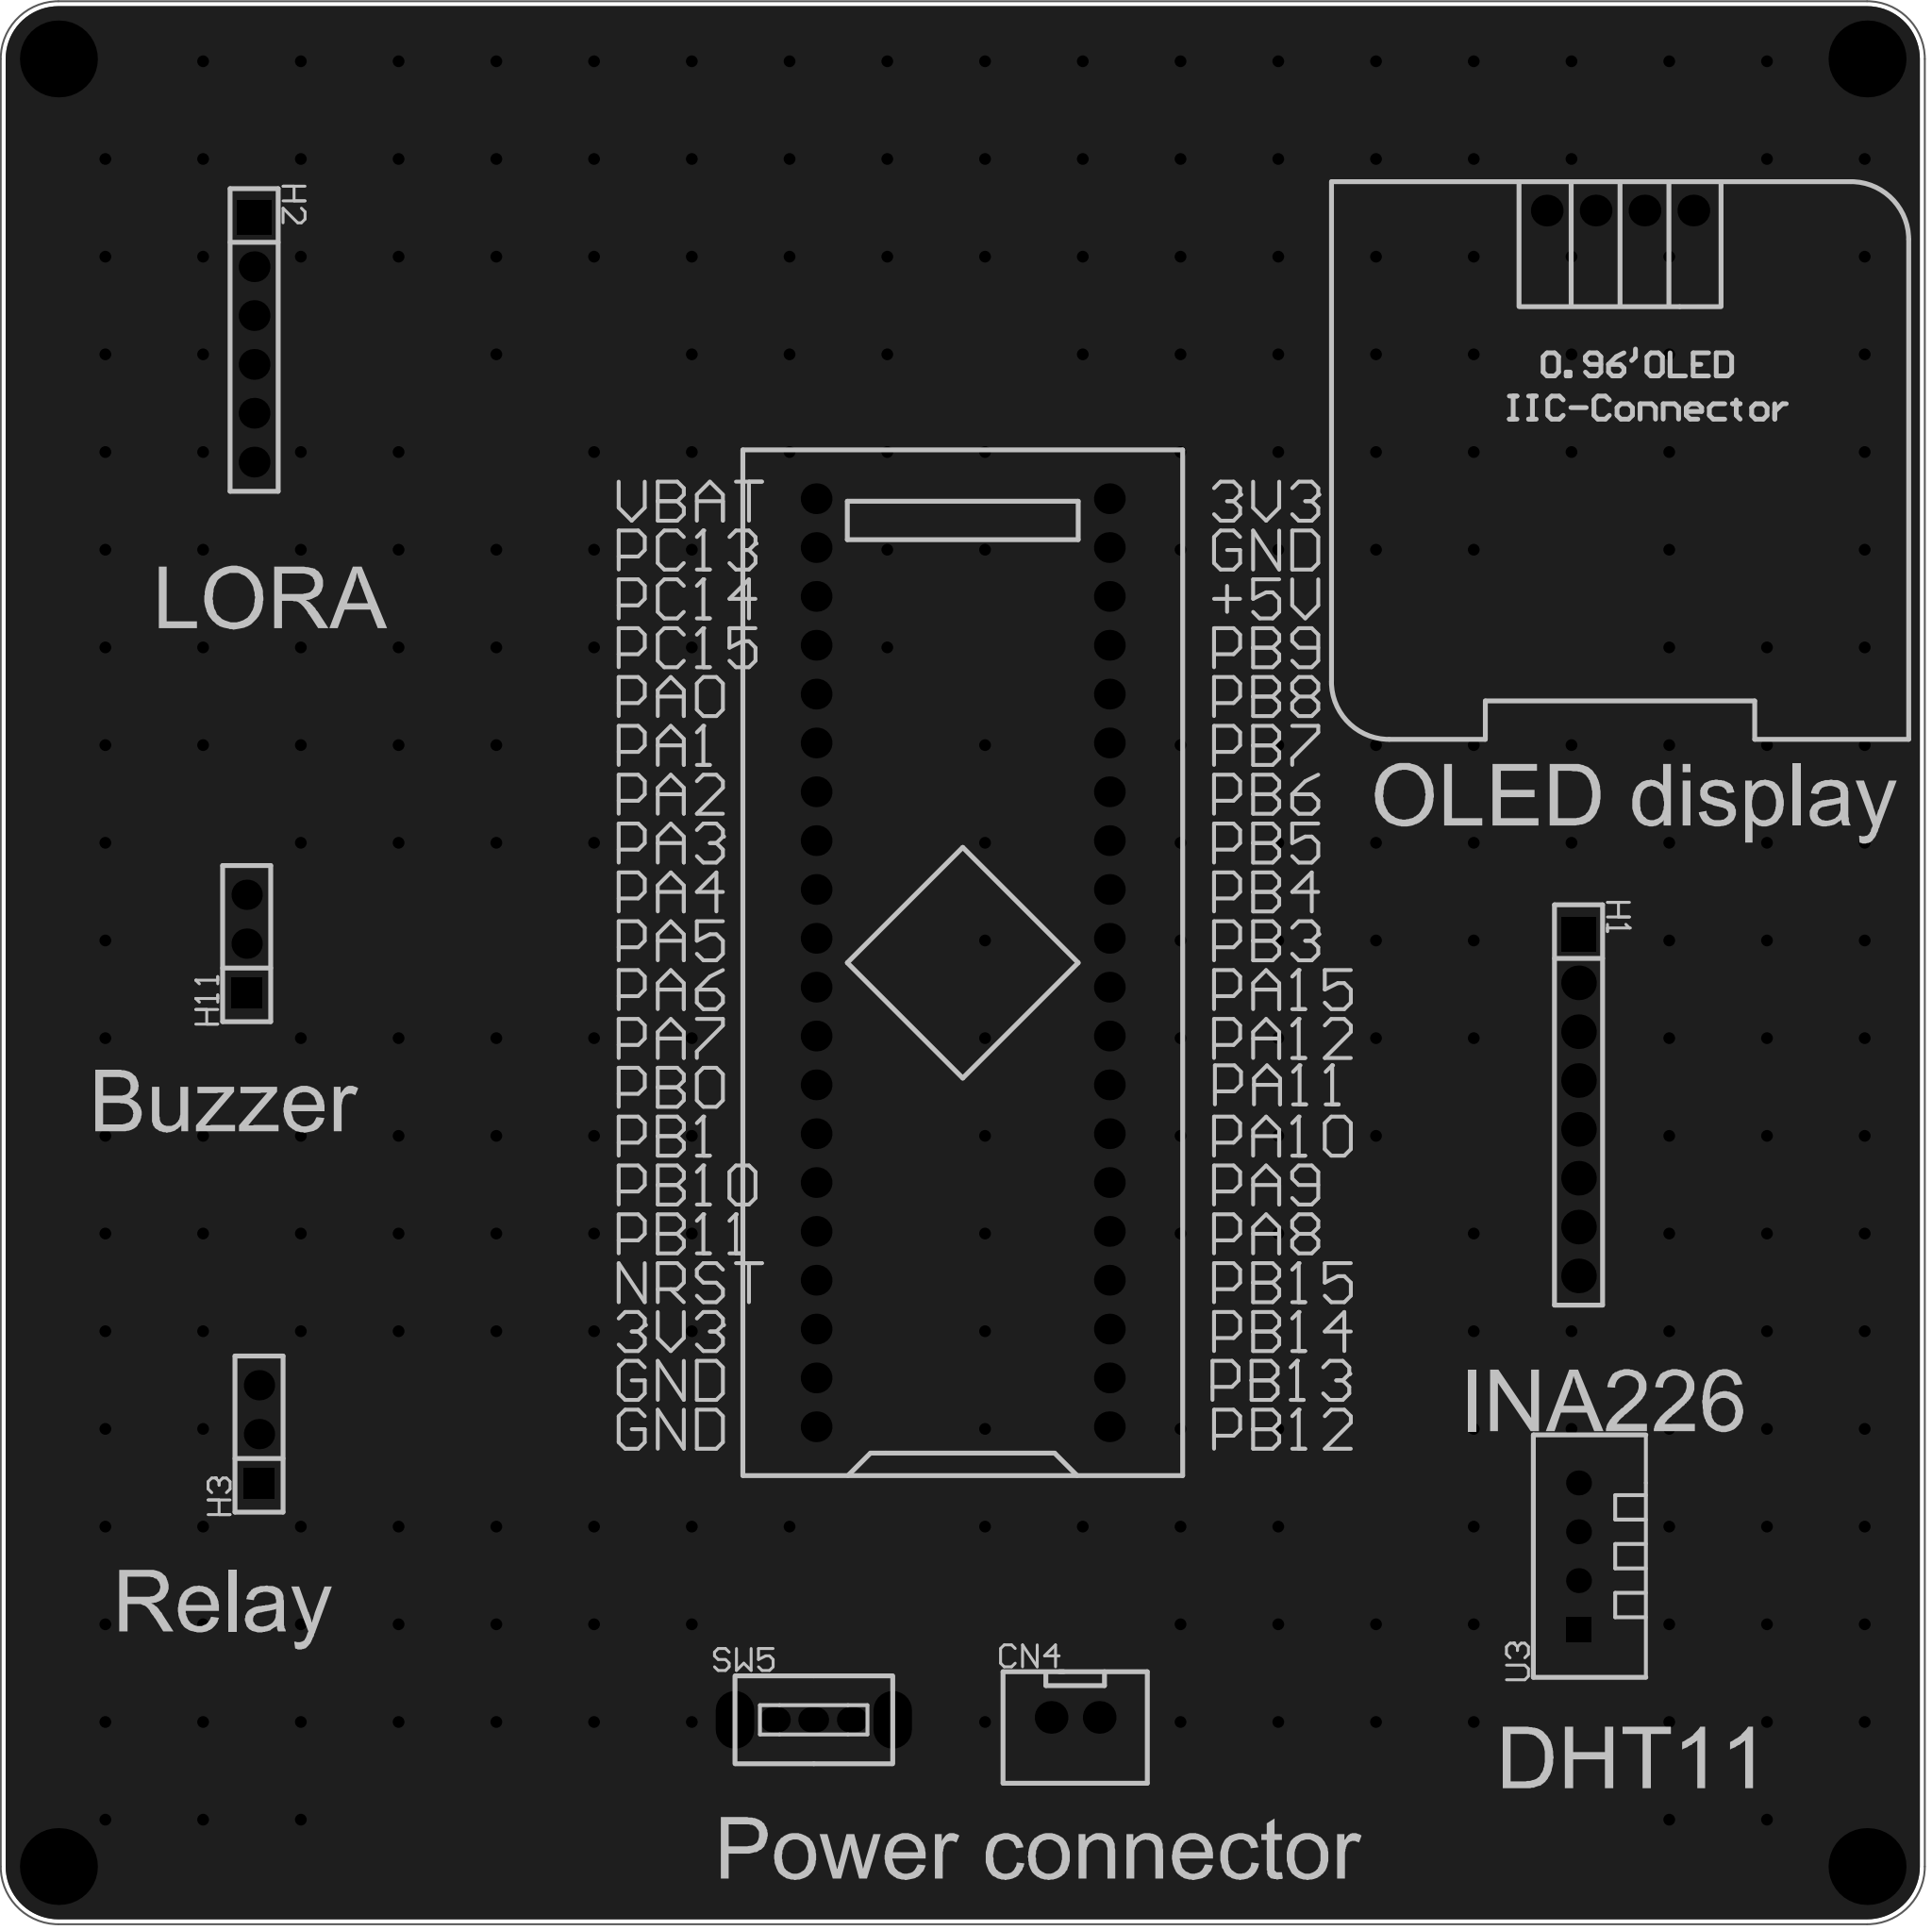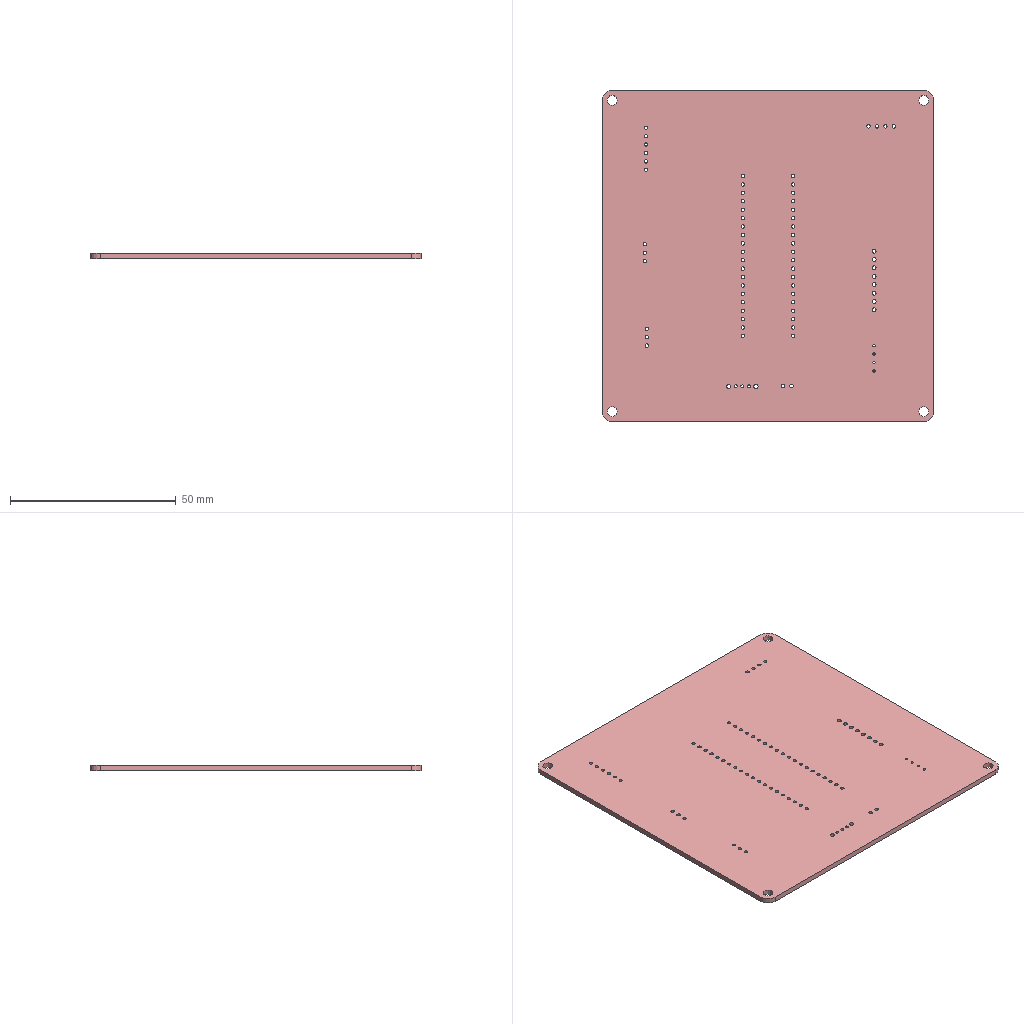Circuit board layout | Altium Designer | box 100 x 100 x 1.6 mm
Layer stack:
# Altium Designer layer stack of  (unit mm; dielectric type: 0 none, 1 core, 2 prepreg, 3 surface material)
index,name,kind,layer,copper_thickness_mm,dielectric_type,dielectric_thickness_mm,dielectric_material,dielectric_constant
0,Top Paste Mask Layer,other,,,,,,
1,Top Silkscreen Layer,other,,,,,,
2,Top Solder Mask Layer,dielectric,,,3,0.01,,3.3
3,Top Layer,copper,Top Layer,0.035,,,,
4,Dielectric1,dielectric,,,3,1.51,FR4,4.5
5,Bottom Layer,copper,Bottom Layer,0.035,,,,
6,Bottom Solder Mask Layer,dielectric,,,3,0.01,,3.3
7,Bottom Silkscreen Layer,other,,,,,,
8,Bottom Paste Mask Layer,other,,,,,,
# drill layer pairs: low layer,high layer
drill_pair,Top Layer,Bottom Layer
Part placement:
Designator,Comment,Layer,Footprint,Center-X(mm),Center-Y(mm),Rotation
U1,STM32F103C8T6-Card,TopLayer,CONN-TH_L53.3-W22.9_STM32F103C8T6-CARD,141.351,130.937,90
OLED1,,TopLayer,0.96OLED_4P,175.514,170.053,0
H11,,TopLayer,HDR-TH_3P-P2.54-V-F,104.133,131.931,90
CN4,XH2.54*2P_Through-hole,TopLayer,CONN-TH_2P-P2.50-XH2.54-2P,147.193,91.694,0
SW5,,TopLayer,拨动开关,133.612,91.567,0
H3,,TopLayer,HDR-TH_3P-P2.54-V-F,104.775,106.426,90
H1,,TopLayer,HDR-TH_8P-P2.54-V-F-1,173.355,123.541,270
H2,,TopLayer,HDR-TH_6P-P2.54-V-F,104.521,163.322,270
U3,DHT11,TopLayer,SENSOR-TH_DHT11,173.355,100.076,90
Pad and via stacks:
# Altium Designer via and pad stacks of  (unit mm). Each distinct definition once, with the count of objects using it.
# via: kind,start_layer,end_layer,hole_mm,diameter_mm,mode(0 simple;1 top-mid-bottom;2 full stack),diameter_per_layer,count,example_net
# pad: kind,layer,hole_mm,hole_type(0 round;1 square;2 slot),plating,top_size,top_shape(1 round;2 rect;3 octagon;9 rounded rect),mid_size,bottom_size,mode,footprint,size_per_layer,count,example
pad,Multi-Layer,3,0,plated,4x4,1,4x4,4x4,0,,,4,1
pad,Multi-Layer,1,0,plated,1.6x1.6,1,1.6x1.6,1.6x1.6,0,CONN-TH_L53.3-W22.9_STM32F103C8T6-CARD,,40,U1.1
pad,Multi-Layer,1,0,plated,1.65x1.65,1,1.65x1.65,1.65x1.65,0,0.96OLED_4P,,4,OLED1.4
pad,Multi-Layer,1.02,0,plated,1.575x1.575,1,1.575x1.575,1.575x1.575,0,HDR-TH_3P-P2.54-V-F,,4,H11.3
pad,Multi-Layer,1.02,0,plated,1.575x1.575,2,1.575x1.575,1.575x1.575,0,HDR-TH_3P-P2.54-V-F,,2,H11.1
pad,Multi-Layer,1.05,0,plated,1.7x1.7,1,1.7x1.7,1.7x1.7,0,CONN-TH_2P-P2.50-XH2.54-2P,,2,CN4.2
pad,Multi-Layer,0.8992,0,plated,1.6x1.3,1,1.6x1.3,1.6x1.3,0,\u00B2\u00A6\u00B6\u00AF\u00BF\u00AA\u00B9\u00D8,,3,SW5.1
pad,Multi-Layer,1.3,0,plated,3x1.999,1,3x1.999,3x1.999,0,\u00B2\u00A6\u00B6\u00AF\u00BF\u00AA\u00B9\u00D8,,2,SW5.4
pad,Multi-Layer,1.2,0,plated,1.8x1.8,2,1.8x1.8,1.8x1.8,0,HDR-TH_8P-P2.54-V-F-1,,1,H1.1
pad,Multi-Layer,1.2,0,plated,1.8x1.8,1,1.8x1.8,1.8x1.8,0,HDR-TH_8P-P2.54-V-F-1,,7,H1.2
pad,Multi-Layer,1.02,0,plated,1.6x1.6,1,1.6x1.6,1.6x1.6,0,HDR-TH_6P-P2.54-V-F,,5,H2.6
pad,Multi-Layer,1.02,0,plated,1.8x1.8,2,1.8x1.8,1.8x1.8,0,HDR-TH_6P-P2.54-V-F,,1,H2.1
pad,Multi-Layer,0.7112,0,plated,1.295x1.295,2,1.295x1.295,1.295x1.295,0,SENSOR-TH_DHT11,,1,U3.1
pad,Multi-Layer,0.7112,0,plated,1.295x1.295,1,1.295x1.295,1.295x1.295,0,SENSOR-TH_DHT11,,3,U3.2
via,Top Layer,Bottom Layer,0.3048,0.61,0,,261,GND
Copper pours:
name,layer,net,type(0 solid;1 hatched;2 none)
Bottom Layer-GND,Bottom Layer,GND,0
Top Layer-GND,Top Layer,GND,0